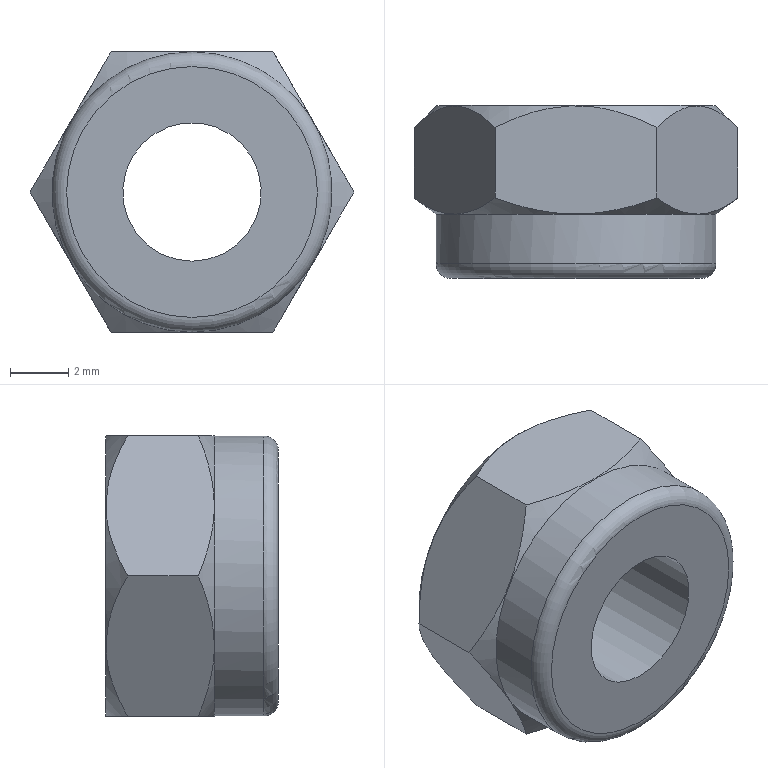Part | NX | features solid 2 | 1 solid | 13 faces | box 11.145 x 5.944 x 9.652 mm | volume 351.738 mm3 | plane 8 | cone 2 | cylinder 2 | torus 1 | commonest cylinder face diameters 4.763 x1 9.632 x1
STEP:
#1=CARTESIAN_POINT('',(0.,2.244,-4.816));
#2=VERTEX_POINT('',#1);
#3=CARTESIAN_POINT('',(0.,2.244,0.));
#4=DIRECTION('',(0.,-1.,0.));
#5=DIRECTION('',(0.,0.,-1.));
#6=AXIS2_PLACEMENT_3D('',#3,#4,#5);
#7=CIRCLE('',#6,4.816);
#8=EDGE_CURVE('',#2,#2,#7,.T.);
#9=ORIENTED_EDGE('',*,*,#8,.F.);
#10=EDGE_LOOP('',(#9));
#11=FACE_BOUND('',#10,.T.);
#12=CARTESIAN_POINT('',(2.786,2.799,-4.826));
#13=VERTEX_POINT('',#12);
#14=CARTESIAN_POINT('',(-2.786,2.799,-4.826));
#15=VERTEX_POINT('',#14);
#16=CARTESIAN_POINT('',(-2.786,2.799,-4.826));
#17=CARTESIAN_POINT('',(-1.894,2.472,-4.826));
#18=CARTESIAN_POINT('',(-0.01026,2.031,-4.826));
#19=CARTESIAN_POINT('',(1.888,2.469,-4.826));
#20=CARTESIAN_POINT('',(2.786,2.799,-4.826));
#21=B_SPLINE_CURVE_WITH_KNOTS('',3,(#16,#17,#18,#19,#20),.UNSPECIFIED.,.F.,.F.,(4,1,4),(0.004401,0.007239,0.01008),.UNSPECIFIED.);
#22=EDGE_CURVE('',#13,#15,#21,.F.);
#23=ORIENTED_EDGE('',*,*,#22,.F.);
#24=CARTESIAN_POINT('',(5.573,2.799,0.));
#25=VERTEX_POINT('',#24);
#26=CARTESIAN_POINT('',(5.573,2.799,0.));
#27=CARTESIAN_POINT('',(5.123,2.469,-0.7782));
#28=CARTESIAN_POINT('',(4.192,2.033,-2.392));
#29=CARTESIAN_POINT('',(3.237,2.468,-4.045));
#30=CARTESIAN_POINT('',(2.786,2.799,-4.826));
#31=B_SPLINE_CURVE_WITH_KNOTS('',3,(#26,#27,#28,#29,#30),.UNSPECIFIED.,.F.,.F.,(4,1,4),(0.000000242,0.002827,0.005653),.UNSPECIFIED.);
#32=EDGE_CURVE('',#25,#13,#31,.T.);
#33=ORIENTED_EDGE('',*,*,#32,.F.);
#34=CARTESIAN_POINT('',(2.786,2.799,4.826));
#35=VERTEX_POINT('',#34);
#36=CARTESIAN_POINT('',(2.786,2.799,4.826));
#37=CARTESIAN_POINT('',(3.236,2.469,4.048));
#38=CARTESIAN_POINT('',(4.167,2.033,2.434));
#39=CARTESIAN_POINT('',(5.122,2.468,0.7809));
#40=CARTESIAN_POINT('',(5.573,2.799,0.));
#41=B_SPLINE_CURVE_WITH_KNOTS('',3,(#36,#37,#38,#39,#40),.UNSPECIFIED.,.F.,.F.,(4,1,4),(0.000000242,0.002827,0.005653),.UNSPECIFIED.);
#42=EDGE_CURVE('',#35,#25,#41,.T.);
#43=ORIENTED_EDGE('',*,*,#42,.F.);
#44=CARTESIAN_POINT('',(-2.786,2.799,4.826));
#45=VERTEX_POINT('',#44);
#46=CARTESIAN_POINT('',(-2.786,2.799,4.826));
#47=CARTESIAN_POINT('',(-1.894,2.472,4.826));
#48=CARTESIAN_POINT('',(-0.01026,2.031,4.826));
#49=CARTESIAN_POINT('',(1.888,2.469,4.826));
#50=CARTESIAN_POINT('',(2.786,2.799,4.826));
#51=B_SPLINE_CURVE_WITH_KNOTS('',3,(#46,#47,#48,#49,#50),.UNSPECIFIED.,.F.,.F.,(4,1,4),(0.004401,0.007239,0.01008),.UNSPECIFIED.);
#52=EDGE_CURVE('',#45,#35,#51,.T.);
#53=ORIENTED_EDGE('',*,*,#52,.F.);
#54=CARTESIAN_POINT('',(-5.573,2.799,0.));
#55=VERTEX_POINT('',#54);
#56=CARTESIAN_POINT('',(-5.573,2.799,0.));
#57=CARTESIAN_POINT('',(-5.123,2.469,0.7782));
#58=CARTESIAN_POINT('',(-4.192,2.033,2.392));
#59=CARTESIAN_POINT('',(-3.237,2.468,4.045));
#60=CARTESIAN_POINT('',(-2.786,2.799,4.826));
#61=B_SPLINE_CURVE_WITH_KNOTS('',3,(#56,#57,#58,#59,#60),.UNSPECIFIED.,.F.,.F.,(4,1,4),(0.000000242,0.002827,0.005653),.UNSPECIFIED.);
#62=EDGE_CURVE('',#55,#45,#61,.T.);
#63=ORIENTED_EDGE('',*,*,#62,.F.);
#64=CARTESIAN_POINT('',(-2.786,2.799,-4.826));
#65=CARTESIAN_POINT('',(-3.236,2.469,-4.048));
#66=CARTESIAN_POINT('',(-4.167,2.033,-2.434));
#67=CARTESIAN_POINT('',(-5.122,2.468,-0.7809));
#68=CARTESIAN_POINT('',(-5.573,2.799,0.));
#69=B_SPLINE_CURVE_WITH_KNOTS('',3,(#64,#65,#66,#67,#68),.UNSPECIFIED.,.F.,.F.,(4,1,4),(0.000000242,0.002827,0.005653),.UNSPECIFIED.);
#70=EDGE_CURVE('',#15,#55,#69,.T.);
#71=ORIENTED_EDGE('',*,*,#70,.F.);
#72=EDGE_LOOP('',(#23,#33,#43,#53,#63,#71));
#73=FACE_BOUND('',#72,.T.);
#74=CARTESIAN_POINT('',(0.,2.244,0.));
#75=DIRECTION('',(0.,1.,0.));
#76=DIRECTION('',(0.,0.,1.));
#77=AXIS2_PLACEMENT_3D('',#74,#75,#76);
#78=CONICAL_SURFACE('',#77,4.816,0.9373);
#79=ADVANCED_FACE('',(#11,#73),#78,.T.);
#80=CARTESIAN_POINT('',(0.,5.987,-4.816));
#81=VERTEX_POINT('',#80);
#82=CARTESIAN_POINT('',(0.,5.987,0.));
#83=DIRECTION('',(0.,-1.,0.));
#84=DIRECTION('',(0.,0.,-1.));
#85=AXIS2_PLACEMENT_3D('',#82,#83,#84);
#86=CIRCLE('',#85,4.816);
#87=EDGE_CURVE('',#81,#81,#86,.T.);
#88=ORIENTED_EDGE('',*,*,#87,.T.);
#89=EDGE_LOOP('',(#88));
#90=FACE_BOUND('',#89,.T.);
#91=CARTESIAN_POINT('',(-2.786,5.231,-4.826));
#92=VERTEX_POINT('',#91);
#93=CARTESIAN_POINT('',(2.786,5.231,-4.826));
#94=VERTEX_POINT('',#93);
#95=CARTESIAN_POINT('',(-2.786,5.231,-4.826));
#96=CARTESIAN_POINT('',(-1.921,5.663,-4.826));
#97=CARTESIAN_POINT('',(0.00213,6.292,-4.826));
#98=CARTESIAN_POINT('',(1.924,5.662,-4.826));
#99=CARTESIAN_POINT('',(2.786,5.231,-4.826));
#100=B_SPLINE_CURVE_WITH_KNOTS('',3,(#95,#96,#97,#98,#99),.UNSPECIFIED.,.F.,.F.,(4,1,4),(0.003774,0.006663,0.009552),.UNSPECIFIED.);
#101=EDGE_CURVE('',#92,#94,#100,.T.);
#102=ORIENTED_EDGE('',*,*,#101,.F.);
#103=CARTESIAN_POINT('',(-5.573,5.231,0.));
#104=VERTEX_POINT('',#103);
#105=CARTESIAN_POINT('',(-5.573,5.231,0.));
#106=CARTESIAN_POINT('',(-5.137,5.666,-0.7541));
#107=CARTESIAN_POINT('',(-4.188,6.287,-2.397));
#108=CARTESIAN_POINT('',(-3.224,5.669,-4.067));
#109=CARTESIAN_POINT('',(-2.786,5.231,-4.826));
#110=B_SPLINE_CURVE_WITH_KNOTS('',3,(#105,#106,#107,#108,#109),.UNSPECIFIED.,.F.,.F.,(4,1,4),(0.000000254,0.002878,0.005757),.UNSPECIFIED.);
#111=EDGE_CURVE('',#104,#92,#110,.T.);
#112=ORIENTED_EDGE('',*,*,#111,.F.);
#113=CARTESIAN_POINT('',(-2.786,5.231,4.826));
#114=VERTEX_POINT('',#113);
#115=CARTESIAN_POINT('',(-2.786,5.231,4.826));
#116=CARTESIAN_POINT('',(-3.222,5.666,4.072));
#117=CARTESIAN_POINT('',(-4.17,6.287,2.429));
#118=CARTESIAN_POINT('',(-5.135,5.669,0.7586));
#119=CARTESIAN_POINT('',(-5.573,5.231,0.));
#120=B_SPLINE_CURVE_WITH_KNOTS('',3,(#115,#116,#117,#118,#119),.UNSPECIFIED.,.F.,.F.,(4,1,4),(0.000000254,0.002878,0.005757),.UNSPECIFIED.);
#121=EDGE_CURVE('',#114,#104,#120,.T.);
#122=ORIENTED_EDGE('',*,*,#121,.F.);
#123=CARTESIAN_POINT('',(2.786,5.231,4.826));
#124=VERTEX_POINT('',#123);
#125=CARTESIAN_POINT('',(-2.786,5.231,4.826));
#126=CARTESIAN_POINT('',(-1.921,5.663,4.826));
#127=CARTESIAN_POINT('',(0.00213,6.292,4.826));
#128=CARTESIAN_POINT('',(1.924,5.662,4.826));
#129=CARTESIAN_POINT('',(2.786,5.231,4.826));
#130=B_SPLINE_CURVE_WITH_KNOTS('',3,(#125,#126,#127,#128,#129),.UNSPECIFIED.,.F.,.F.,(4,1,4),(0.003774,0.006663,0.009552),.UNSPECIFIED.);
#131=EDGE_CURVE('',#124,#114,#130,.F.);
#132=ORIENTED_EDGE('',*,*,#131,.F.);
#133=CARTESIAN_POINT('',(5.573,5.231,0.));
#134=VERTEX_POINT('',#133);
#135=CARTESIAN_POINT('',(5.573,5.231,0.));
#136=CARTESIAN_POINT('',(5.137,5.666,0.7541));
#137=CARTESIAN_POINT('',(4.188,6.287,2.397));
#138=CARTESIAN_POINT('',(3.224,5.669,4.067));
#139=CARTESIAN_POINT('',(2.786,5.231,4.826));
#140=B_SPLINE_CURVE_WITH_KNOTS('',3,(#135,#136,#137,#138,#139),.UNSPECIFIED.,.F.,.F.,(4,1,4),(0.000000254,0.002878,0.005757),.UNSPECIFIED.);
#141=EDGE_CURVE('',#134,#124,#140,.T.);
#142=ORIENTED_EDGE('',*,*,#141,.F.);
#143=CARTESIAN_POINT('',(2.786,5.231,-4.826));
#144=CARTESIAN_POINT('',(3.222,5.666,-4.072));
#145=CARTESIAN_POINT('',(4.17,6.287,-2.429));
#146=CARTESIAN_POINT('',(5.135,5.669,-0.7586));
#147=CARTESIAN_POINT('',(5.573,5.231,0.));
#148=B_SPLINE_CURVE_WITH_KNOTS('',3,(#143,#144,#145,#146,#147),.UNSPECIFIED.,.F.,.F.,(4,1,4),(0.000000254,0.002878,0.005757),.UNSPECIFIED.);
#149=EDGE_CURVE('',#94,#134,#148,.T.);
#150=ORIENTED_EDGE('',*,*,#149,.F.);
#151=EDGE_LOOP('',(#102,#112,#122,#132,#142,#150));
#152=FACE_BOUND('',#151,.T.);
#153=CARTESIAN_POINT('',(0.,5.422,0.));
#154=DIRECTION('',(0.,-1.,0.));
#155=DIRECTION('',(0.,0.,-1.));
#156=AXIS2_PLACEMENT_3D('',#153,#154,#155);
#157=CONICAL_SURFACE('',#156,5.382,0.7854);
#158=ADVANCED_FACE('',(#90,#152),#157,.T.);
#159=CARTESIAN_POINT('',(0.,5.987,-2.381));
#160=VERTEX_POINT('',#159);
#161=CARTESIAN_POINT('',(0.,5.987,0.));
#162=DIRECTION('',(0.,-1.,0.));
#163=DIRECTION('',(0.,0.,-1.));
#164=AXIS2_PLACEMENT_3D('',#161,#162,#163);
#165=CIRCLE('',#164,2.381);
#166=EDGE_CURVE('',#160,#160,#165,.T.);
#167=ORIENTED_EDGE('',*,*,#166,.T.);
#168=EDGE_LOOP('',(#167));
#169=FACE_BOUND('',#168,.T.);
#170=ORIENTED_EDGE('',*,*,#87,.F.);
#171=EDGE_LOOP('',(#170));
#172=FACE_BOUND('',#171,.T.);
#173=CARTESIAN_POINT('',(0.,5.987,4.816));
#174=DIRECTION('',(0.,1.,0.));
#175=DIRECTION('',(0.,0.,1.));
#176=AXIS2_PLACEMENT_3D('',#173,#174,#175);
#177=PLANE('',#176);
#178=ADVANCED_FACE('',(#169,#172),#177,.T.);
#179=CARTESIAN_POINT('',(0.,0.0436,-2.381));
#180=VERTEX_POINT('',#179);
#181=CARTESIAN_POINT('',(0.,0.0436,0.));
#182=DIRECTION('',(0.,-1.,0.));
#183=DIRECTION('',(0.,0.,-1.));
#184=AXIS2_PLACEMENT_3D('',#181,#182,#183);
#185=CIRCLE('',#184,2.381);
#186=EDGE_CURVE('',#180,#180,#185,.T.);
#187=ORIENTED_EDGE('',*,*,#186,.T.);
#188=EDGE_LOOP('',(#187));
#189=FACE_BOUND('',#188,.T.);
#190=ORIENTED_EDGE('',*,*,#166,.F.);
#191=EDGE_LOOP('',(#190));
#192=FACE_BOUND('',#191,.T.);
#193=CARTESIAN_POINT('',(0.,0.,0.));
#194=DIRECTION('',(0.,-1.,0.));
#195=DIRECTION('',(0.,0.,-1.));
#196=AXIS2_PLACEMENT_3D('',#193,#194,#195);
#197=CYLINDRICAL_SURFACE('',#196,2.381);
#198=ADVANCED_FACE('',(#189,#192),#197,.F.);
#199=CARTESIAN_POINT('',(0.,0.0436,-4.316));
#200=VERTEX_POINT('',#199);
#201=CARTESIAN_POINT('',(0.,0.0436,0.));
#202=DIRECTION('',(0.,-1.,0.));
#203=DIRECTION('',(0.,0.,-1.));
#204=AXIS2_PLACEMENT_3D('',#201,#202,#203);
#205=CIRCLE('',#204,4.316);
#206=EDGE_CURVE('',#200,#200,#205,.T.);
#207=ORIENTED_EDGE('',*,*,#206,.T.);
#208=EDGE_LOOP('',(#207));
#209=FACE_BOUND('',#208,.T.);
#210=ORIENTED_EDGE('',*,*,#186,.F.);
#211=EDGE_LOOP('',(#210));
#212=FACE_BOUND('',#211,.T.);
#213=CARTESIAN_POINT('',(0.,0.0436,2.381));
#214=DIRECTION('',(0.,-1.,0.));
#215=DIRECTION('',(0.,0.,-1.));
#216=AXIS2_PLACEMENT_3D('',#213,#214,#215);
#217=PLANE('',#216);
#218=ADVANCED_FACE('',(#209,#212),#217,.T.);
#219=CARTESIAN_POINT('',(0.,0.5436,-4.816));
#220=VERTEX_POINT('',#219);
#221=CARTESIAN_POINT('',(0.,0.5436,0.));
#222=DIRECTION('',(0.,-1.,0.));
#223=DIRECTION('',(0.,0.,-1.));
#224=AXIS2_PLACEMENT_3D('',#221,#222,#223);
#225=CIRCLE('',#224,4.816);
#226=EDGE_CURVE('',#220,#220,#225,.F.);
#227=ORIENTED_EDGE('',*,*,#226,.T.);
#228=EDGE_LOOP('',(#227));
#229=FACE_BOUND('',#228,.T.);
#230=ORIENTED_EDGE('',*,*,#8,.T.);
#231=EDGE_LOOP('',(#230));
#232=FACE_BOUND('',#231,.T.);
#233=CARTESIAN_POINT('',(0.,0.,0.));
#234=DIRECTION('',(0.,-1.,0.));
#235=DIRECTION('',(0.,0.,-1.));
#236=AXIS2_PLACEMENT_3D('',#233,#234,#235);
#237=CYLINDRICAL_SURFACE('',#236,4.816);
#238=ADVANCED_FACE('',(#229,#232),#237,.T.);
#239=CARTESIAN_POINT('',(2.786,42.,-4.826));
#240=DIRECTION('',(0.,-1.,0.));
#241=VECTOR('',#240,1000.);
#242=LINE('',#239,#241);
#243=EDGE_CURVE('',#94,#13,#242,.T.);
#244=ORIENTED_EDGE('',*,*,#243,.T.);
#245=ORIENTED_EDGE('',*,*,#22,.T.);
#246=CARTESIAN_POINT('',(-2.786,42.,-4.826));
#247=DIRECTION('',(0.,-1.,0.));
#248=VECTOR('',#247,1000.);
#249=LINE('',#246,#248);
#250=EDGE_CURVE('',#92,#15,#249,.T.);
#251=ORIENTED_EDGE('',*,*,#250,.F.);
#252=ORIENTED_EDGE('',*,*,#101,.T.);
#253=EDGE_LOOP('',(#244,#245,#251,#252));
#254=FACE_BOUND('',#253,.T.);
#255=CARTESIAN_POINT('',(2.786,42.,-4.826));
#256=DIRECTION('',(0.,0.,1.));
#257=DIRECTION('',(1.,0.,0.));
#258=AXIS2_PLACEMENT_3D('',#255,#256,#257);
#259=PLANE('',#258);
#260=ADVANCED_FACE('',(#254),#259,.F.);
#261=ORIENTED_EDGE('',*,*,#250,.T.);
#262=ORIENTED_EDGE('',*,*,#70,.T.);
#263=CARTESIAN_POINT('',(-5.573,42.,0.));
#264=DIRECTION('',(0.,-1.,0.));
#265=VECTOR('',#264,1000.);
#266=LINE('',#263,#265);
#267=EDGE_CURVE('',#104,#55,#266,.T.);
#268=ORIENTED_EDGE('',*,*,#267,.F.);
#269=ORIENTED_EDGE('',*,*,#111,.T.);
#270=EDGE_LOOP('',(#261,#262,#268,#269));
#271=FACE_BOUND('',#270,.T.);
#272=CARTESIAN_POINT('',(-2.786,42.,-4.826));
#273=DIRECTION('',(0.866,0.,0.5));
#274=DIRECTION('',(0.5,0.,-0.866));
#275=AXIS2_PLACEMENT_3D('',#272,#273,#274);
#276=PLANE('',#275);
#277=ADVANCED_FACE('',(#271),#276,.F.);
#278=ORIENTED_EDGE('',*,*,#267,.T.);
#279=ORIENTED_EDGE('',*,*,#62,.T.);
#280=CARTESIAN_POINT('',(-2.786,42.,4.826));
#281=DIRECTION('',(0.,-1.,0.));
#282=VECTOR('',#281,1000.);
#283=LINE('',#280,#282);
#284=EDGE_CURVE('',#114,#45,#283,.T.);
#285=ORIENTED_EDGE('',*,*,#284,.F.);
#286=ORIENTED_EDGE('',*,*,#121,.T.);
#287=EDGE_LOOP('',(#278,#279,#285,#286));
#288=FACE_BOUND('',#287,.T.);
#289=CARTESIAN_POINT('',(-5.573,42.,0.));
#290=DIRECTION('',(0.866,0.,-0.5));
#291=DIRECTION('',(-0.5,0.,-0.866));
#292=AXIS2_PLACEMENT_3D('',#289,#290,#291);
#293=PLANE('',#292);
#294=ADVANCED_FACE('',(#288),#293,.F.);
#295=ORIENTED_EDGE('',*,*,#284,.T.);
#296=ORIENTED_EDGE('',*,*,#52,.T.);
#297=CARTESIAN_POINT('',(2.786,42.,4.826));
#298=DIRECTION('',(0.,-1.,0.));
#299=VECTOR('',#298,1000.);
#300=LINE('',#297,#299);
#301=EDGE_CURVE('',#124,#35,#300,.T.);
#302=ORIENTED_EDGE('',*,*,#301,.F.);
#303=ORIENTED_EDGE('',*,*,#131,.T.);
#304=EDGE_LOOP('',(#295,#296,#302,#303));
#305=FACE_BOUND('',#304,.T.);
#306=CARTESIAN_POINT('',(-2.786,42.,4.826));
#307=DIRECTION('',(0.,0.,-1.));
#308=DIRECTION('',(-1.,0.,0.));
#309=AXIS2_PLACEMENT_3D('',#306,#307,#308);
#310=PLANE('',#309);
#311=ADVANCED_FACE('',(#305),#310,.F.);
#312=ORIENTED_EDGE('',*,*,#301,.T.);
#313=ORIENTED_EDGE('',*,*,#42,.T.);
#314=CARTESIAN_POINT('',(5.573,42.,0.));
#315=DIRECTION('',(0.,-1.,0.));
#316=VECTOR('',#315,1000.);
#317=LINE('',#314,#316);
#318=EDGE_CURVE('',#134,#25,#317,.T.);
#319=ORIENTED_EDGE('',*,*,#318,.F.);
#320=ORIENTED_EDGE('',*,*,#141,.T.);
#321=EDGE_LOOP('',(#312,#313,#319,#320));
#322=FACE_BOUND('',#321,.T.);
#323=CARTESIAN_POINT('',(2.786,42.,4.826));
#324=DIRECTION('',(-0.866,0.,-0.5));
#325=DIRECTION('',(-0.5,0.,0.866));
#326=AXIS2_PLACEMENT_3D('',#323,#324,#325);
#327=PLANE('',#326);
#328=ADVANCED_FACE('',(#322),#327,.F.);
#329=ORIENTED_EDGE('',*,*,#318,.T.);
#330=ORIENTED_EDGE('',*,*,#32,.T.);
#331=ORIENTED_EDGE('',*,*,#243,.F.);
#332=ORIENTED_EDGE('',*,*,#149,.T.);
#333=EDGE_LOOP('',(#329,#330,#331,#332));
#334=FACE_BOUND('',#333,.T.);
#335=CARTESIAN_POINT('',(5.573,42.,0.));
#336=DIRECTION('',(-0.866,0.,0.5));
#337=DIRECTION('',(0.5,0.,0.866));
#338=AXIS2_PLACEMENT_3D('',#335,#336,#337);
#339=PLANE('',#338);
#340=ADVANCED_FACE('',(#334),#339,.F.);
#341=ORIENTED_EDGE('',*,*,#226,.F.);
#342=EDGE_LOOP('',(#341));
#343=FACE_BOUND('',#342,.T.);
#344=ORIENTED_EDGE('',*,*,#206,.F.);
#345=EDGE_LOOP('',(#344));
#346=FACE_BOUND('',#345,.T.);
#347=CARTESIAN_POINT('',(0.,0.5436,0.));
#348=DIRECTION('',(0.,-1.,0.));
#349=DIRECTION('',(0.,0.,-1.));
#350=AXIS2_PLACEMENT_3D('',#347,#348,#349);
#351=TOROIDAL_SURFACE('',#350,4.316,0.5);
#352=ADVANCED_FACE('',(#343,#346),#351,.T.);
#353=CLOSED_SHELL('',(#79,#158,#178,#198,#218,#238,#260,#277,#294,#311,#328,#340,#352));
#354=MANIFOLD_SOLID_BREP('',#353);
#355=(LENGTH_UNIT()NAMED_UNIT(*)SI_UNIT(.MILLI.,.METRE.));
#356=UNCERTAINTY_MEASURE_WITH_UNIT(LENGTH_MEASURE(0.0508),#355,'','');
#357=(NAMED_UNIT(*)PLANE_ANGLE_UNIT()SI_UNIT($,.RADIAN.));
#358=(NAMED_UNIT(*)SI_UNIT($,.STERADIAN.)SOLID_ANGLE_UNIT());
#359=(GEOMETRIC_REPRESENTATION_CONTEXT(3)GLOBAL_UNCERTAINTY_ASSIGNED_CONTEXT((#356))GLOBAL_UNIT_ASSIGNED_CONTEXT((#355,#357,#358))REPRESENTATION_CONTEXT('',''));
#360=ADVANCED_BREP_SHAPE_REPRESENTATION('',(#354),#359);